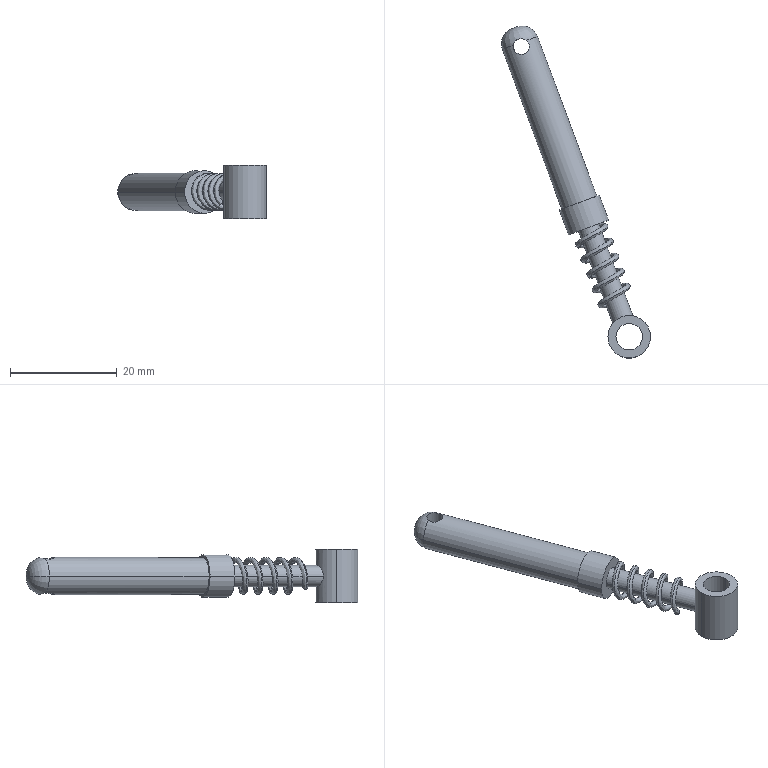Part | SolidWorks | features ICE 4, 3DProfileFeature 2, Extrusion 1, Fillet 1, Helix 1, Sweep 1 | 2 solids | 23 faces | box 27.99 x 62.362 x 10 mm | volume 2119 mm3 | cylinder 12 | plane 7 | torus 2 | spline 2 | commonest cylinder face diameters 8 x4 3 x2 4 x2 5 x2 7 x2